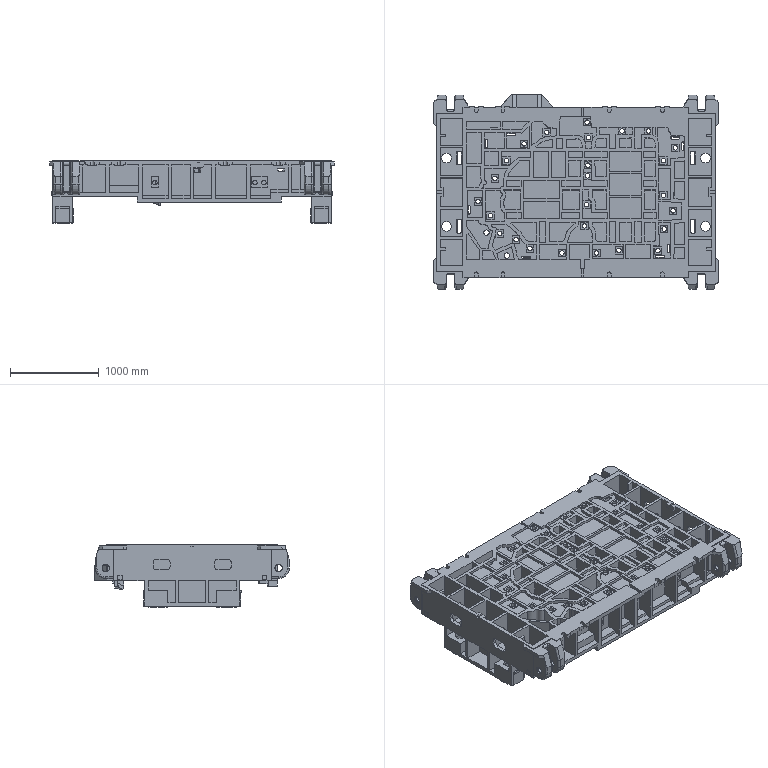Part | NX | features solid 2 | 1 solid | 2505 faces | box 3210 x 2195 x 700 mm | volume 876986173 mm3 | plane 1908 | cylinder 384 | spline 181 | torus 32 | commonest cylinder face diameters 40 x65 20 x55 80 x51 83 x48 10 x34 51 x26